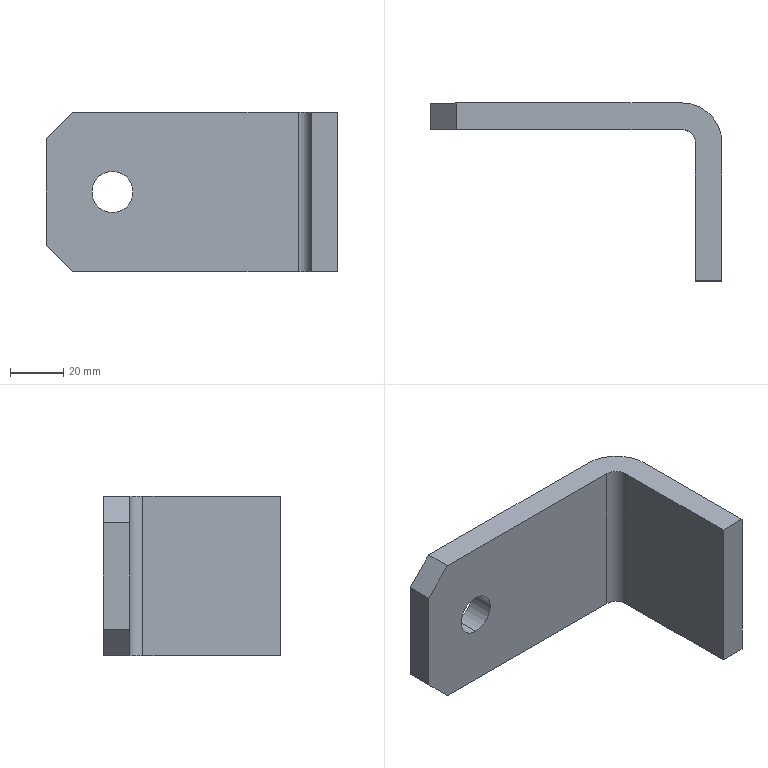Part | SolidWorks | features Chamfer 1, Extrusion 1, HoleWzd 1 | 1 solid | 14 faces | box 110 x 67 x 60 mm | volume 94738 mm3 | plane 10 | cylinder 4 | commonest cylinder face diameters 15.5 x2 10 x1 30 x1
STEP:
#1=CARTESIAN_POINT('',(25.,-10.,22.25));
#2=VERTEX_POINT('',#1);
#3=CARTESIAN_POINT('',(25.,-10.,37.75));
#4=VERTEX_POINT('',#3);
#5=CARTESIAN_POINT('',(25.,-10.,30.));
#6=DIRECTION('',(0.,1.,0.));
#7=DIRECTION('',(0.,0.,1.));
#8=AXIS2_PLACEMENT_3D('',#5,#6,#7);
#9=CIRCLE('',#8,7.75);
#10=EDGE_CURVE('',#2,#4,#9,.T.);
#11=ORIENTED_EDGE('',*,*,#10,.F.);
#12=CARTESIAN_POINT('',(25.,0.,22.25));
#13=VERTEX_POINT('',#12);
#14=CARTESIAN_POINT('',(25.,0.,22.25));
#15=DIRECTION('',(0.,1.,0.));
#16=VECTOR('',#15,1000.);
#17=LINE('',#14,#16);
#18=EDGE_CURVE('',#2,#13,#17,.T.);
#19=ORIENTED_EDGE('',*,*,#18,.T.);
#20=CARTESIAN_POINT('',(25.,0.,37.75));
#21=VERTEX_POINT('',#20);
#22=CARTESIAN_POINT('',(25.,0.,30.));
#23=DIRECTION('',(0.,1.,0.));
#24=DIRECTION('',(0.,0.,1.));
#25=AXIS2_PLACEMENT_3D('',#22,#23,#24);
#26=CIRCLE('',#25,7.75);
#27=EDGE_CURVE('',#13,#21,#26,.T.);
#28=ORIENTED_EDGE('',*,*,#27,.T.);
#29=CARTESIAN_POINT('',(25.,0.,37.75));
#30=DIRECTION('',(0.,1.,0.));
#31=VECTOR('',#30,1000.);
#32=LINE('',#29,#31);
#33=EDGE_CURVE('',#4,#21,#32,.T.);
#34=ORIENTED_EDGE('',*,*,#33,.F.);
#35=EDGE_LOOP('',(#11,#19,#28,#34));
#36=FACE_OUTER_BOUND('',#35,.T.);
#37=CARTESIAN_POINT('',(25.,0.,30.));
#38=DIRECTION('',(0.,1.,0.));
#39=DIRECTION('',(0.,0.,1.));
#40=AXIS2_PLACEMENT_3D('',#37,#38,#39);
#41=CYLINDRICAL_SURFACE('',#40,7.75);
#42=ADVANCED_FACE('',(#36),#41,.F.);
#43=CARTESIAN_POINT('',(0.,0.,50.));
#44=VERTEX_POINT('',#43);
#45=CARTESIAN_POINT('',(0.,0.,10.));
#46=VERTEX_POINT('',#45);
#47=CARTESIAN_POINT('',(0.,0.,60.));
#48=DIRECTION('',(0.,0.,-1.));
#49=VECTOR('',#48,1000.);
#50=LINE('',#47,#49);
#51=EDGE_CURVE('',#44,#46,#50,.T.);
#52=ORIENTED_EDGE('',*,*,#51,.T.);
#53=CARTESIAN_POINT('',(0.,-10.,10.));
#54=VERTEX_POINT('',#53);
#55=CARTESIAN_POINT('',(0.,-10.,10.));
#56=DIRECTION('',(0.,-1.,0.));
#57=VECTOR('',#56,1000.);
#58=LINE('',#55,#57);
#59=EDGE_CURVE('',#46,#54,#58,.T.);
#60=ORIENTED_EDGE('',*,*,#59,.T.);
#61=CARTESIAN_POINT('',(0.,-10.,50.));
#62=VERTEX_POINT('',#61);
#63=CARTESIAN_POINT('',(0.,-10.,60.));
#64=DIRECTION('',(0.,0.,-1.));
#65=VECTOR('',#64,1000.);
#66=LINE('',#63,#65);
#67=EDGE_CURVE('',#62,#54,#66,.T.);
#68=ORIENTED_EDGE('',*,*,#67,.F.);
#69=CARTESIAN_POINT('',(0.,-10.,50.));
#70=DIRECTION('',(0.,1.,0.));
#71=VECTOR('',#70,1000.);
#72=LINE('',#69,#71);
#73=EDGE_CURVE('',#62,#44,#72,.T.);
#74=ORIENTED_EDGE('',*,*,#73,.T.);
#75=EDGE_LOOP('',(#52,#60,#68,#74));
#76=FACE_OUTER_BOUND('',#75,.T.);
#77=CARTESIAN_POINT('',(0.,-10.,60.));
#78=DIRECTION('',(1.,0.,0.));
#79=DIRECTION('',(0.,0.,-1.));
#80=AXIS2_PLACEMENT_3D('',#77,#78,#79);
#81=PLANE('',#80);
#82=ADVANCED_FACE('',(#76),#81,.F.);
#83=CARTESIAN_POINT('',(25.,-10.,30.));
#84=DIRECTION('',(0.,1.,0.));
#85=DIRECTION('',(0.,0.,1.));
#86=AXIS2_PLACEMENT_3D('',#83,#84,#85);
#87=CIRCLE('',#86,7.75);
#88=EDGE_CURVE('',#4,#2,#87,.T.);
#89=ORIENTED_EDGE('',*,*,#88,.T.);
#90=ORIENTED_EDGE('',*,*,#10,.T.);
#91=EDGE_LOOP('',(#89,#90));
#92=FACE_BOUND('',#91,.T.);
#93=ORIENTED_EDGE('',*,*,#67,.T.);
#94=CARTESIAN_POINT('',(10.,-10.,0.));
#95=VERTEX_POINT('',#94);
#96=CARTESIAN_POINT('',(0.,-10.,10.));
#97=DIRECTION('',(0.7071,0.,-0.7071));
#98=VECTOR('',#97,1000.);
#99=LINE('',#96,#98);
#100=EDGE_CURVE('',#54,#95,#99,.T.);
#101=ORIENTED_EDGE('',*,*,#100,.T.);
#102=CARTESIAN_POINT('',(95.,-10.,0.));
#103=VERTEX_POINT('',#102);
#104=CARTESIAN_POINT('',(0.,-10.,0.));
#105=DIRECTION('',(1.,0.,0.));
#106=VECTOR('',#105,1000.);
#107=LINE('',#104,#106);
#108=EDGE_CURVE('',#95,#103,#107,.T.);
#109=ORIENTED_EDGE('',*,*,#108,.T.);
#110=CARTESIAN_POINT('',(95.,-10.,60.));
#111=VERTEX_POINT('',#110);
#112=CARTESIAN_POINT('',(95.,-10.,60.));
#113=DIRECTION('',(0.,0.,-1.));
#114=VECTOR('',#113,1000.);
#115=LINE('',#112,#114);
#116=EDGE_CURVE('',#111,#103,#115,.T.);
#117=ORIENTED_EDGE('',*,*,#116,.F.);
#118=CARTESIAN_POINT('',(10.,-10.,60.));
#119=VERTEX_POINT('',#118);
#120=CARTESIAN_POINT('',(0.,-10.,60.));
#121=DIRECTION('',(1.,0.,0.));
#122=VECTOR('',#121,1000.);
#123=LINE('',#120,#122);
#124=EDGE_CURVE('',#119,#111,#123,.T.);
#125=ORIENTED_EDGE('',*,*,#124,.F.);
#126=CARTESIAN_POINT('',(10.,-10.,60.));
#127=DIRECTION('',(-0.7071,0.,-0.7071));
#128=VECTOR('',#127,1000.);
#129=LINE('',#126,#128);
#130=EDGE_CURVE('',#119,#62,#129,.T.);
#131=ORIENTED_EDGE('',*,*,#130,.T.);
#132=EDGE_LOOP('',(#93,#101,#109,#117,#125,#131));
#133=FACE_OUTER_BOUND('',#132,.T.);
#134=CARTESIAN_POINT('',(0.,-10.,60.));
#135=DIRECTION('',(0.,1.,0.));
#136=DIRECTION('',(0.,0.,1.));
#137=AXIS2_PLACEMENT_3D('',#134,#135,#136);
#138=PLANE('',#137);
#139=ADVANCED_FACE('',(#92,#133),#138,.F.);
#140=CARTESIAN_POINT('',(100.,-15.,0.));
#141=VERTEX_POINT('',#140);
#142=CARTESIAN_POINT('',(95.,-15.,0.));
#143=DIRECTION('',(0.,0.,-1.));
#144=DIRECTION('',(-1.,0.,0.));
#145=AXIS2_PLACEMENT_3D('',#142,#143,#144);
#146=CIRCLE('',#145,5.);
#147=EDGE_CURVE('',#103,#141,#146,.T.);
#148=ORIENTED_EDGE('',*,*,#147,.T.);
#149=CARTESIAN_POINT('',(100.,-15.,60.));
#150=VERTEX_POINT('',#149);
#151=CARTESIAN_POINT('',(100.,-15.,60.));
#152=DIRECTION('',(0.,0.,-1.));
#153=VECTOR('',#152,1000.);
#154=LINE('',#151,#153);
#155=EDGE_CURVE('',#150,#141,#154,.T.);
#156=ORIENTED_EDGE('',*,*,#155,.F.);
#157=CARTESIAN_POINT('',(95.,-15.,60.));
#158=DIRECTION('',(0.,0.,-1.));
#159=DIRECTION('',(-1.,0.,0.));
#160=AXIS2_PLACEMENT_3D('',#157,#158,#159);
#161=CIRCLE('',#160,5.);
#162=EDGE_CURVE('',#111,#150,#161,.T.);
#163=ORIENTED_EDGE('',*,*,#162,.F.);
#164=ORIENTED_EDGE('',*,*,#116,.T.);
#165=EDGE_LOOP('',(#148,#156,#163,#164));
#166=FACE_OUTER_BOUND('',#165,.T.);
#167=CARTESIAN_POINT('',(95.,-15.,60.));
#168=DIRECTION('',(0.,0.,-1.));
#169=DIRECTION('',(-1.,0.,0.));
#170=AXIS2_PLACEMENT_3D('',#167,#168,#169);
#171=CYLINDRICAL_SURFACE('',#170,5.);
#172=ADVANCED_FACE('',(#166),#171,.F.);
#173=CARTESIAN_POINT('',(100.,-67.,0.));
#174=VERTEX_POINT('',#173);
#175=CARTESIAN_POINT('',(100.,-15.,0.));
#176=DIRECTION('',(0.,-1.,0.));
#177=VECTOR('',#176,1000.);
#178=LINE('',#175,#177);
#179=EDGE_CURVE('',#141,#174,#178,.T.);
#180=ORIENTED_EDGE('',*,*,#179,.T.);
#181=CARTESIAN_POINT('',(100.,-67.,60.));
#182=VERTEX_POINT('',#181);
#183=CARTESIAN_POINT('',(100.,-67.,60.));
#184=DIRECTION('',(0.,0.,-1.));
#185=VECTOR('',#184,1000.);
#186=LINE('',#183,#185);
#187=EDGE_CURVE('',#182,#174,#186,.T.);
#188=ORIENTED_EDGE('',*,*,#187,.F.);
#189=CARTESIAN_POINT('',(100.,-15.,60.));
#190=DIRECTION('',(0.,-1.,0.));
#191=VECTOR('',#190,1000.);
#192=LINE('',#189,#191);
#193=EDGE_CURVE('',#150,#182,#192,.T.);
#194=ORIENTED_EDGE('',*,*,#193,.F.);
#195=ORIENTED_EDGE('',*,*,#155,.T.);
#196=EDGE_LOOP('',(#180,#188,#194,#195));
#197=FACE_OUTER_BOUND('',#196,.T.);
#198=CARTESIAN_POINT('',(100.,-15.,60.));
#199=DIRECTION('',(1.,0.,0.));
#200=DIRECTION('',(0.,1.,0.));
#201=AXIS2_PLACEMENT_3D('',#198,#199,#200);
#202=PLANE('',#201);
#203=ADVANCED_FACE('',(#197),#202,.F.);
#204=CARTESIAN_POINT('',(110.,-67.,0.));
#205=VERTEX_POINT('',#204);
#206=CARTESIAN_POINT('',(110.,-67.,0.));
#207=DIRECTION('',(1.,0.,0.));
#208=VECTOR('',#207,1000.);
#209=LINE('',#206,#208);
#210=EDGE_CURVE('',#174,#205,#209,.T.);
#211=ORIENTED_EDGE('',*,*,#210,.T.);
#212=CARTESIAN_POINT('',(110.,-67.,60.));
#213=VERTEX_POINT('',#212);
#214=CARTESIAN_POINT('',(110.,-67.,60.));
#215=DIRECTION('',(0.,0.,-1.));
#216=VECTOR('',#215,1000.);
#217=LINE('',#214,#216);
#218=EDGE_CURVE('',#213,#205,#217,.T.);
#219=ORIENTED_EDGE('',*,*,#218,.F.);
#220=CARTESIAN_POINT('',(110.,-67.,60.));
#221=DIRECTION('',(1.,0.,0.));
#222=VECTOR('',#221,1000.);
#223=LINE('',#220,#222);
#224=EDGE_CURVE('',#182,#213,#223,.T.);
#225=ORIENTED_EDGE('',*,*,#224,.F.);
#226=ORIENTED_EDGE('',*,*,#187,.T.);
#227=EDGE_LOOP('',(#211,#219,#225,#226));
#228=FACE_OUTER_BOUND('',#227,.T.);
#229=CARTESIAN_POINT('',(110.,-67.,60.));
#230=DIRECTION('',(0.,1.,0.));
#231=DIRECTION('',(0.,0.,1.));
#232=AXIS2_PLACEMENT_3D('',#229,#230,#231);
#233=PLANE('',#232);
#234=ADVANCED_FACE('',(#228),#233,.F.);
#235=CARTESIAN_POINT('',(110.,-15.,0.));
#236=VERTEX_POINT('',#235);
#237=CARTESIAN_POINT('',(110.,-15.,0.));
#238=DIRECTION('',(0.,1.,0.));
#239=VECTOR('',#238,1000.);
#240=LINE('',#237,#239);
#241=EDGE_CURVE('',#205,#236,#240,.T.);
#242=ORIENTED_EDGE('',*,*,#241,.T.);
#243=CARTESIAN_POINT('',(110.,-15.,60.));
#244=VERTEX_POINT('',#243);
#245=CARTESIAN_POINT('',(110.,-15.,60.));
#246=DIRECTION('',(0.,0.,-1.));
#247=VECTOR('',#246,1000.);
#248=LINE('',#245,#247);
#249=EDGE_CURVE('',#244,#236,#248,.T.);
#250=ORIENTED_EDGE('',*,*,#249,.F.);
#251=CARTESIAN_POINT('',(110.,-15.,60.));
#252=DIRECTION('',(0.,1.,0.));
#253=VECTOR('',#252,1000.);
#254=LINE('',#251,#253);
#255=EDGE_CURVE('',#213,#244,#254,.T.);
#256=ORIENTED_EDGE('',*,*,#255,.F.);
#257=ORIENTED_EDGE('',*,*,#218,.T.);
#258=EDGE_LOOP('',(#242,#250,#256,#257));
#259=FACE_OUTER_BOUND('',#258,.T.);
#260=CARTESIAN_POINT('',(110.,-15.,60.));
#261=DIRECTION('',(-1.,0.,0.));
#262=DIRECTION('',(0.,-1.,0.));
#263=AXIS2_PLACEMENT_3D('',#260,#261,#262);
#264=PLANE('',#263);
#265=ADVANCED_FACE('',(#259),#264,.F.);
#266=CARTESIAN_POINT('',(95.,0.,0.));
#267=VERTEX_POINT('',#266);
#268=CARTESIAN_POINT('',(95.,-15.,0.));
#269=DIRECTION('',(0.,0.,1.));
#270=DIRECTION('',(-1.,0.,0.));
#271=AXIS2_PLACEMENT_3D('',#268,#269,#270);
#272=CIRCLE('',#271,15.);
#273=EDGE_CURVE('',#236,#267,#272,.T.);
#274=ORIENTED_EDGE('',*,*,#273,.T.);
#275=CARTESIAN_POINT('',(95.,0.,60.));
#276=VERTEX_POINT('',#275);
#277=CARTESIAN_POINT('',(95.,0.,60.));
#278=DIRECTION('',(0.,0.,-1.));
#279=VECTOR('',#278,1000.);
#280=LINE('',#277,#279);
#281=EDGE_CURVE('',#276,#267,#280,.T.);
#282=ORIENTED_EDGE('',*,*,#281,.F.);
#283=CARTESIAN_POINT('',(95.,-15.,60.));
#284=DIRECTION('',(0.,0.,1.));
#285=DIRECTION('',(-1.,0.,0.));
#286=AXIS2_PLACEMENT_3D('',#283,#284,#285);
#287=CIRCLE('',#286,15.);
#288=EDGE_CURVE('',#244,#276,#287,.T.);
#289=ORIENTED_EDGE('',*,*,#288,.F.);
#290=ORIENTED_EDGE('',*,*,#249,.T.);
#291=EDGE_LOOP('',(#274,#282,#289,#290));
#292=FACE_OUTER_BOUND('',#291,.T.);
#293=CARTESIAN_POINT('',(95.,-15.,60.));
#294=DIRECTION('',(0.,0.,-1.));
#295=DIRECTION('',(-1.,0.,0.));
#296=AXIS2_PLACEMENT_3D('',#293,#294,#295);
#297=CYLINDRICAL_SURFACE('',#296,15.);
#298=ADVANCED_FACE('',(#292),#297,.T.);
#299=CARTESIAN_POINT('',(25.,0.,30.));
#300=DIRECTION('',(0.,1.,0.));
#301=DIRECTION('',(0.,0.,1.));
#302=AXIS2_PLACEMENT_3D('',#299,#300,#301);
#303=CIRCLE('',#302,7.75);
#304=EDGE_CURVE('',#21,#13,#303,.T.);
#305=ORIENTED_EDGE('',*,*,#304,.F.);
#306=ORIENTED_EDGE('',*,*,#27,.F.);
#307=EDGE_LOOP('',(#305,#306));
#308=FACE_BOUND('',#307,.T.);
#309=CARTESIAN_POINT('',(10.,0.,0.));
#310=VERTEX_POINT('',#309);
#311=CARTESIAN_POINT('',(0.,0.,0.));
#312=DIRECTION('',(-1.,0.,0.));
#313=VECTOR('',#312,1000.);
#314=LINE('',#311,#313);
#315=EDGE_CURVE('',#267,#310,#314,.T.);
#316=ORIENTED_EDGE('',*,*,#315,.T.);
#317=CARTESIAN_POINT('',(0.,0.,10.));
#318=DIRECTION('',(-0.7071,0.,0.7071));
#319=VECTOR('',#318,1000.);
#320=LINE('',#317,#319);
#321=EDGE_CURVE('',#310,#46,#320,.T.);
#322=ORIENTED_EDGE('',*,*,#321,.T.);
#323=ORIENTED_EDGE('',*,*,#51,.F.);
#324=CARTESIAN_POINT('',(10.,0.,60.));
#325=VERTEX_POINT('',#324);
#326=CARTESIAN_POINT('',(10.,0.,60.));
#327=DIRECTION('',(0.7071,0.,0.7071));
#328=VECTOR('',#327,1000.);
#329=LINE('',#326,#328);
#330=EDGE_CURVE('',#44,#325,#329,.T.);
#331=ORIENTED_EDGE('',*,*,#330,.T.);
#332=CARTESIAN_POINT('',(0.,0.,60.));
#333=DIRECTION('',(-1.,0.,0.));
#334=VECTOR('',#333,1000.);
#335=LINE('',#332,#334);
#336=EDGE_CURVE('',#276,#325,#335,.T.);
#337=ORIENTED_EDGE('',*,*,#336,.F.);
#338=ORIENTED_EDGE('',*,*,#281,.T.);
#339=EDGE_LOOP('',(#316,#322,#323,#331,#337,#338));
#340=FACE_OUTER_BOUND('',#339,.T.);
#341=CARTESIAN_POINT('',(0.,0.,60.));
#342=DIRECTION('',(0.,-1.,0.));
#343=DIRECTION('',(0.,0.,-1.));
#344=AXIS2_PLACEMENT_3D('',#341,#342,#343);
#345=PLANE('',#344);
#346=ADVANCED_FACE('',(#308,#340),#345,.F.);
#347=ORIENTED_EDGE('',*,*,#336,.T.);
#348=CARTESIAN_POINT('',(10.,-15.,60.));
#349=DIRECTION('',(0.,-1.,0.));
#350=VECTOR('',#349,1000.);
#351=LINE('',#348,#350);
#352=EDGE_CURVE('',#325,#119,#351,.T.);
#353=ORIENTED_EDGE('',*,*,#352,.T.);
#354=ORIENTED_EDGE('',*,*,#124,.T.);
#355=ORIENTED_EDGE('',*,*,#162,.T.);
#356=ORIENTED_EDGE('',*,*,#193,.T.);
#357=ORIENTED_EDGE('',*,*,#224,.T.);
#358=ORIENTED_EDGE('',*,*,#255,.T.);
#359=ORIENTED_EDGE('',*,*,#288,.T.);
#360=EDGE_LOOP('',(#347,#353,#354,#355,#356,#357,#358,#359));
#361=FACE_OUTER_BOUND('',#360,.T.);
#362=CARTESIAN_POINT('',(95.,-15.,60.));
#363=DIRECTION('',(0.,0.,-1.));
#364=DIRECTION('',(-1.,0.,0.));
#365=AXIS2_PLACEMENT_3D('',#362,#363,#364);
#366=PLANE('',#365);
#367=ADVANCED_FACE('',(#361),#366,.F.);
#368=ORIENTED_EDGE('',*,*,#108,.F.);
#369=CARTESIAN_POINT('',(10.,0.,0.));
#370=DIRECTION('',(0.,1.,0.));
#371=VECTOR('',#370,1000.);
#372=LINE('',#369,#371);
#373=EDGE_CURVE('',#95,#310,#372,.T.);
#374=ORIENTED_EDGE('',*,*,#373,.T.);
#375=ORIENTED_EDGE('',*,*,#315,.F.);
#376=ORIENTED_EDGE('',*,*,#273,.F.);
#377=ORIENTED_EDGE('',*,*,#241,.F.);
#378=ORIENTED_EDGE('',*,*,#210,.F.);
#379=ORIENTED_EDGE('',*,*,#179,.F.);
#380=ORIENTED_EDGE('',*,*,#147,.F.);
#381=EDGE_LOOP('',(#368,#374,#375,#376,#377,#378,#379,#380));
#382=FACE_OUTER_BOUND('',#381,.T.);
#383=CARTESIAN_POINT('',(95.,-15.,0.));
#384=DIRECTION('',(0.,0.,-1.));
#385=DIRECTION('',(-1.,0.,0.));
#386=AXIS2_PLACEMENT_3D('',#383,#384,#385);
#387=PLANE('',#386);
#388=ADVANCED_FACE('',(#382),#387,.T.);
#389=ORIENTED_EDGE('',*,*,#321,.F.);
#390=ORIENTED_EDGE('',*,*,#373,.F.);
#391=ORIENTED_EDGE('',*,*,#100,.F.);
#392=ORIENTED_EDGE('',*,*,#59,.F.);
#393=EDGE_LOOP('',(#389,#390,#391,#392));
#394=FACE_OUTER_BOUND('',#393,.T.);
#395=CARTESIAN_POINT('',(0.,-10.,10.));
#396=DIRECTION('',(-0.7071,0.,-0.7071));
#397=DIRECTION('',(0.,1.,0.));
#398=AXIS2_PLACEMENT_3D('',#395,#396,#397);
#399=PLANE('',#398);
#400=ADVANCED_FACE('',(#394),#399,.T.);
#401=ORIENTED_EDGE('',*,*,#330,.F.);
#402=ORIENTED_EDGE('',*,*,#73,.F.);
#403=ORIENTED_EDGE('',*,*,#130,.F.);
#404=ORIENTED_EDGE('',*,*,#352,.F.);
#405=EDGE_LOOP('',(#401,#402,#403,#404));
#406=FACE_OUTER_BOUND('',#405,.T.);
#407=CARTESIAN_POINT('',(10.,-15.,60.));
#408=DIRECTION('',(0.7071,0.,-0.7071));
#409=DIRECTION('',(0.,-1.,0.));
#410=AXIS2_PLACEMENT_3D('',#407,#408,#409);
#411=PLANE('',#410);
#412=ADVANCED_FACE('',(#406),#411,.F.);
#413=ORIENTED_EDGE('',*,*,#18,.F.);
#414=ORIENTED_EDGE('',*,*,#88,.F.);
#415=ORIENTED_EDGE('',*,*,#33,.T.);
#416=ORIENTED_EDGE('',*,*,#304,.T.);
#417=EDGE_LOOP('',(#413,#414,#415,#416));
#418=FACE_OUTER_BOUND('',#417,.T.);
#419=CARTESIAN_POINT('',(25.,0.,30.));
#420=DIRECTION('',(0.,1.,0.));
#421=DIRECTION('',(0.,0.,1.));
#422=AXIS2_PLACEMENT_3D('',#419,#420,#421);
#423=CYLINDRICAL_SURFACE('',#422,7.75);
#424=ADVANCED_FACE('',(#418),#423,.F.);
#425=CLOSED_SHELL('',(#42,#82,#139,#172,#203,#234,#265,#298,#346,#367,#388,#400,#412,#424));
#426=MANIFOLD_SOLID_BREP('',#425);
#427=CARTESIAN_POINT('',(0.,0.,0.));
#428=DIRECTION('',(0.,0.,1.));
#429=DIRECTION('',(1.,0.,0.));
#430=AXIS2_PLACEMENT_3D('',#427,#428,#429);
#431=(LENGTH_UNIT()NAMED_UNIT(*)SI_UNIT(.MILLI.,.METRE.));
#432=UNCERTAINTY_MEASURE_WITH_UNIT(LENGTH_MEASURE(0.00001),#431,'','');
#433=(NAMED_UNIT(*)PLANE_ANGLE_UNIT()SI_UNIT($,.RADIAN.));
#434=(NAMED_UNIT(*)SI_UNIT($,.STERADIAN.)SOLID_ANGLE_UNIT());
#435=(GEOMETRIC_REPRESENTATION_CONTEXT(3)GLOBAL_UNCERTAINTY_ASSIGNED_CONTEXT((#432))GLOBAL_UNIT_ASSIGNED_CONTEXT((#431,#433,#434))REPRESENTATION_CONTEXT('',''));
#436=ADVANCED_BREP_SHAPE_REPRESENTATION('',(#426,#430),#435);